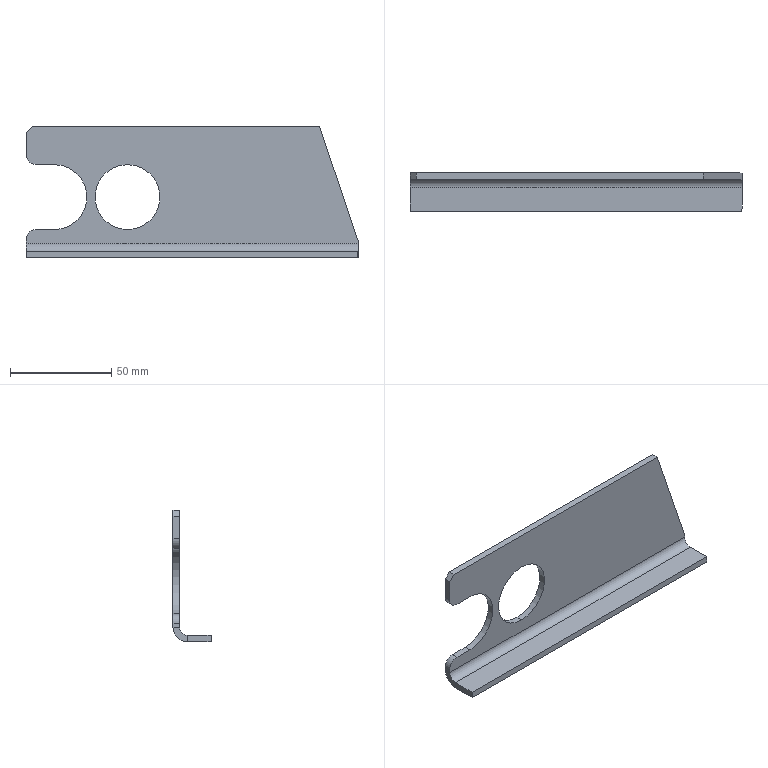Part | SolidWorks | features ICE 3, Fillet 2, BreakCorner 1, EdgeFlange 1, FlatPattern 1, SMBaseFlange 1, SheetMetal 1 | 1 solid | 25 faces | box 163.6 x 18.8 x 65 mm | volume 33886 mm3 | plane 17 | cylinder 8 | commonest cylinder face diameters 32 x3 10 x2 8 x1 14.4 x1 24 x1
STEP:
#1=CARTESIAN_POINT('',(-31.8,-3.2,-18.5));
#2=VERTEX_POINT('',#1);
#3=CARTESIAN_POINT('',(-31.8,-3.2,13.5));
#4=VERTEX_POINT('',#3);
#5=CARTESIAN_POINT('',(-31.8,-3.2,-2.5));
#6=DIRECTION('',(0.,1.,0.));
#7=DIRECTION('',(0.,0.,1.));
#8=AXIS2_PLACEMENT_3D('',#5,#6,#7);
#9=CIRCLE('',#8,16.);
#10=EDGE_CURVE('',#2,#4,#9,.T.);
#11=ORIENTED_EDGE('',*,*,#10,.F.);
#12=CARTESIAN_POINT('',(-31.8,0.,-18.5));
#13=VERTEX_POINT('',#12);
#14=CARTESIAN_POINT('',(-31.8,-10.,-18.5));
#15=DIRECTION('',(0.,1.,0.));
#16=VECTOR('',#15,1000.);
#17=LINE('',#14,#16);
#18=EDGE_CURVE('',#2,#13,#17,.T.);
#19=ORIENTED_EDGE('',*,*,#18,.T.);
#20=CARTESIAN_POINT('',(-31.8,0.,13.5));
#21=VERTEX_POINT('',#20);
#22=CARTESIAN_POINT('',(-31.8,0.,-2.5));
#23=DIRECTION('',(0.,1.,0.));
#24=DIRECTION('',(0.,0.,1.));
#25=AXIS2_PLACEMENT_3D('',#22,#23,#24);
#26=CIRCLE('',#25,16.);
#27=EDGE_CURVE('',#13,#21,#26,.T.);
#28=ORIENTED_EDGE('',*,*,#27,.T.);
#29=CARTESIAN_POINT('',(-31.8,-10.,13.5));
#30=DIRECTION('',(0.,1.,0.));
#31=VECTOR('',#30,1000.);
#32=LINE('',#29,#31);
#33=EDGE_CURVE('',#4,#21,#32,.T.);
#34=ORIENTED_EDGE('',*,*,#33,.F.);
#35=EDGE_LOOP('',(#11,#19,#28,#34));
#36=FACE_OUTER_BOUND('',#35,.T.);
#37=CARTESIAN_POINT('',(-31.8,-10.,-2.5));
#38=DIRECTION('',(0.,1.,0.));
#39=DIRECTION('',(0.,0.,1.));
#40=AXIS2_PLACEMENT_3D('',#37,#38,#39);
#41=CYLINDRICAL_SURFACE('',#40,16.);
#42=ADVANCED_FACE('',(#36),#41,.F.);
#43=CARTESIAN_POINT('',(81.8,0.,-23.7));
#44=VERTEX_POINT('',#43);
#45=CARTESIAN_POINT('',(81.8,0.,-25.3));
#46=VERTEX_POINT('',#45);
#47=CARTESIAN_POINT('',(81.8,0.,-32.5));
#48=DIRECTION('',(0.,0.,-1.));
#49=VECTOR('',#48,1000.);
#50=LINE('',#47,#49);
#51=EDGE_CURVE('',#44,#46,#50,.T.);
#52=ORIENTED_EDGE('',*,*,#51,.F.);
#53=CARTESIAN_POINT('',(81.8,-3.2,-23.7));
#54=VERTEX_POINT('',#53);
#55=CARTESIAN_POINT('',(81.8,0.,-23.7));
#56=DIRECTION('',(0.,-1.,0.));
#57=VECTOR('',#56,1000.);
#58=LINE('',#55,#57);
#59=EDGE_CURVE('',#44,#54,#58,.T.);
#60=ORIENTED_EDGE('',*,*,#59,.T.);
#61=CARTESIAN_POINT('',(81.8,-3.2,-25.3));
#62=VERTEX_POINT('',#61);
#63=CARTESIAN_POINT('',(81.8,-3.2,-32.5));
#64=DIRECTION('',(0.,0.,-1.));
#65=VECTOR('',#64,1000.);
#66=LINE('',#63,#65);
#67=EDGE_CURVE('',#54,#62,#66,.T.);
#68=ORIENTED_EDGE('',*,*,#67,.T.);
#69=CARTESIAN_POINT('',(81.8,-3.2,-25.3));
#70=DIRECTION('',(0.,1.,0.));
#71=VECTOR('',#70,1000.);
#72=LINE('',#69,#71);
#73=EDGE_CURVE('',#62,#46,#72,.T.);
#74=ORIENTED_EDGE('',*,*,#73,.T.);
#75=EDGE_LOOP('',(#52,#60,#68,#74));
#76=FACE_OUTER_BOUND('',#75,.T.);
#77=CARTESIAN_POINT('',(81.8,-3.2,-32.5));
#78=DIRECTION('',(1.,0.,0.));
#79=DIRECTION('',(0.,0.,-1.));
#80=AXIS2_PLACEMENT_3D('',#77,#78,#79);
#81=PLANE('',#80);
#82=ADVANCED_FACE('',(#76),#81,.T.);
#83=CARTESIAN_POINT('',(-31.8,-3.2,-2.5));
#84=DIRECTION('',(0.,1.,0.));
#85=DIRECTION('',(0.,0.,1.));
#86=AXIS2_PLACEMENT_3D('',#83,#84,#85);
#87=CIRCLE('',#86,16.);
#88=EDGE_CURVE('',#4,#2,#87,.T.);
#89=ORIENTED_EDGE('',*,*,#88,.T.);
#90=ORIENTED_EDGE('',*,*,#10,.T.);
#91=EDGE_LOOP('',(#89,#90));
#92=FACE_BOUND('',#91,.T.);
#93=CARTESIAN_POINT('',(-78.8,-3.2,32.5));
#94=VERTEX_POINT('',#93);
#95=CARTESIAN_POINT('',(62.8,-3.2,32.5));
#96=VERTEX_POINT('',#95);
#97=CARTESIAN_POINT('',(-81.8,-3.2,32.5));
#98=DIRECTION('',(1.,0.,0.));
#99=VECTOR('',#98,1000.);
#100=LINE('',#97,#99);
#101=EDGE_CURVE('',#94,#96,#100,.T.);
#102=ORIENTED_EDGE('',*,*,#101,.F.);
#103=CARTESIAN_POINT('',(-81.8,-3.2,29.5));
#104=VERTEX_POINT('',#103);
#105=CARTESIAN_POINT('',(-81.8,-3.2,29.5));
#106=DIRECTION('',(-0.7071,0.,-0.7071));
#107=VECTOR('',#106,1000.);
#108=LINE('',#105,#107);
#109=EDGE_CURVE('',#94,#104,#108,.T.);
#110=ORIENTED_EDGE('',*,*,#109,.T.);
#111=CARTESIAN_POINT('',(-81.8,-3.2,18.5));
#112=VERTEX_POINT('',#111);
#113=CARTESIAN_POINT('',(-81.8,-3.2,-32.5));
#114=DIRECTION('',(0.,0.,1.));
#115=VECTOR('',#114,1000.);
#116=LINE('',#113,#115);
#117=EDGE_CURVE('',#112,#104,#116,.T.);
#118=ORIENTED_EDGE('',*,*,#117,.F.);
#119=CARTESIAN_POINT('',(-76.8,-3.2,13.5));
#120=VERTEX_POINT('',#119);
#121=CARTESIAN_POINT('',(-76.8,-3.2,18.5));
#122=DIRECTION('',(0.,-1.,0.));
#123=DIRECTION('',(0.,0.,1.));
#124=AXIS2_PLACEMENT_3D('',#121,#122,#123);
#125=CIRCLE('',#124,5.);
#126=EDGE_CURVE('',#112,#120,#125,.T.);
#127=ORIENTED_EDGE('',*,*,#126,.T.);
#128=CARTESIAN_POINT('',(-67.8,-3.2,13.5));
#129=VERTEX_POINT('',#128);
#130=CARTESIAN_POINT('',(0.,-3.2,13.5));
#131=DIRECTION('',(1.,0.,0.));
#132=VECTOR('',#131,1000.);
#133=LINE('',#130,#132);
#134=EDGE_CURVE('',#120,#129,#133,.T.);
#135=ORIENTED_EDGE('',*,*,#134,.T.);
#136=CARTESIAN_POINT('',(-67.8,-3.2,-18.5));
#137=VERTEX_POINT('',#136);
#138=CARTESIAN_POINT('',(-67.8,-3.2,-2.5));
#139=DIRECTION('',(0.,1.,0.));
#140=DIRECTION('',(0.,0.,1.));
#141=AXIS2_PLACEMENT_3D('',#138,#139,#140);
#142=CIRCLE('',#141,16.);
#143=EDGE_CURVE('',#129,#137,#142,.T.);
#144=ORIENTED_EDGE('',*,*,#143,.T.);
#145=CARTESIAN_POINT('',(-76.8,-3.2,-18.5));
#146=VERTEX_POINT('',#145);
#147=CARTESIAN_POINT('',(0.,-3.2,-18.5));
#148=DIRECTION('',(-1.,0.,0.));
#149=VECTOR('',#148,1000.);
#150=LINE('',#147,#149);
#151=EDGE_CURVE('',#137,#146,#150,.T.);
#152=ORIENTED_EDGE('',*,*,#151,.T.);
#153=CARTESIAN_POINT('',(-81.8,-3.2,-23.5));
#154=VERTEX_POINT('',#153);
#155=CARTESIAN_POINT('',(-76.8,-3.2,-23.5));
#156=DIRECTION('',(0.,-1.,0.));
#157=DIRECTION('',(0.,0.,1.));
#158=AXIS2_PLACEMENT_3D('',#155,#156,#157);
#159=CIRCLE('',#158,5.);
#160=EDGE_CURVE('',#146,#154,#159,.T.);
#161=ORIENTED_EDGE('',*,*,#160,.T.);
#162=CARTESIAN_POINT('',(-81.8,-3.2,-25.3));
#163=VERTEX_POINT('',#162);
#164=CARTESIAN_POINT('',(-81.8,-3.2,-32.5));
#165=DIRECTION('',(0.,0.,1.));
#166=VECTOR('',#165,1000.);
#167=LINE('',#164,#166);
#168=EDGE_CURVE('',#163,#154,#167,.T.);
#169=ORIENTED_EDGE('',*,*,#168,.F.);
#170=CARTESIAN_POINT('',(81.8,-3.2,-25.3));
#171=DIRECTION('',(-1.,0.,0.));
#172=VECTOR('',#171,1000.);
#173=LINE('',#170,#172);
#174=EDGE_CURVE('',#62,#163,#173,.T.);
#175=ORIENTED_EDGE('',*,*,#174,.F.);
#176=ORIENTED_EDGE('',*,*,#67,.F.);
#177=CARTESIAN_POINT('',(66.219,-3.2,22.387));
#178=DIRECTION('',(0.3203,0.,-0.9473));
#179=VECTOR('',#178,1000.);
#180=LINE('',#177,#179);
#181=EDGE_CURVE('',#96,#54,#180,.T.);
#182=ORIENTED_EDGE('',*,*,#181,.F.);
#183=EDGE_LOOP('',(#102,#110,#118,#127,#135,#144,#152,#161,#169,#175,#176,#182));
#184=FACE_OUTER_BOUND('',#183,.T.);
#185=CARTESIAN_POINT('',(0.,-3.2,0.));
#186=DIRECTION('',(0.,1.,0.));
#187=DIRECTION('',(0.,0.,1.));
#188=AXIS2_PLACEMENT_3D('',#185,#186,#187);
#189=PLANE('',#188);
#190=ADVANCED_FACE('',(#92,#184),#189,.F.);
#191=CARTESIAN_POINT('',(-31.8,0.,-2.5));
#192=DIRECTION('',(0.,1.,0.));
#193=DIRECTION('',(0.,0.,1.));
#194=AXIS2_PLACEMENT_3D('',#191,#192,#193);
#195=CIRCLE('',#194,16.);
#196=EDGE_CURVE('',#21,#13,#195,.T.);
#197=ORIENTED_EDGE('',*,*,#196,.F.);
#198=ORIENTED_EDGE('',*,*,#27,.F.);
#199=EDGE_LOOP('',(#197,#198));
#200=FACE_BOUND('',#199,.T.);
#201=CARTESIAN_POINT('',(-81.8,0.,18.5));
#202=VERTEX_POINT('',#201);
#203=CARTESIAN_POINT('',(-81.8,0.,29.5));
#204=VERTEX_POINT('',#203);
#205=CARTESIAN_POINT('',(-81.8,0.,-32.5));
#206=DIRECTION('',(0.,0.,1.));
#207=VECTOR('',#206,1000.);
#208=LINE('',#205,#207);
#209=EDGE_CURVE('',#202,#204,#208,.T.);
#210=ORIENTED_EDGE('',*,*,#209,.T.);
#211=CARTESIAN_POINT('',(-78.8,0.,32.5));
#212=VERTEX_POINT('',#211);
#213=CARTESIAN_POINT('',(-55.65,0.,55.65));
#214=DIRECTION('',(0.7071,0.,0.7071));
#215=VECTOR('',#214,1000.);
#216=LINE('',#213,#215);
#217=EDGE_CURVE('',#204,#212,#216,.T.);
#218=ORIENTED_EDGE('',*,*,#217,.T.);
#219=CARTESIAN_POINT('',(62.8,0.,32.5));
#220=VERTEX_POINT('',#219);
#221=CARTESIAN_POINT('',(-81.8,0.,32.5));
#222=DIRECTION('',(1.,0.,0.));
#223=VECTOR('',#222,1000.);
#224=LINE('',#221,#223);
#225=EDGE_CURVE('',#212,#220,#224,.T.);
#226=ORIENTED_EDGE('',*,*,#225,.T.);
#227=CARTESIAN_POINT('',(66.219,0.,22.387));
#228=DIRECTION('',(0.3203,0.,-0.9473));
#229=VECTOR('',#228,1000.);
#230=LINE('',#227,#229);
#231=EDGE_CURVE('',#220,#44,#230,.T.);
#232=ORIENTED_EDGE('',*,*,#231,.T.);
#233=ORIENTED_EDGE('',*,*,#51,.T.);
#234=CARTESIAN_POINT('',(-81.8,0.,-25.3));
#235=VERTEX_POINT('',#234);
#236=CARTESIAN_POINT('',(81.8,0.,-25.3));
#237=DIRECTION('',(-1.,0.,0.));
#238=VECTOR('',#237,1000.);
#239=LINE('',#236,#238);
#240=EDGE_CURVE('',#46,#235,#239,.T.);
#241=ORIENTED_EDGE('',*,*,#240,.T.);
#242=CARTESIAN_POINT('',(-81.8,0.,-23.5));
#243=VERTEX_POINT('',#242);
#244=CARTESIAN_POINT('',(-81.8,0.,-32.5));
#245=DIRECTION('',(0.,0.,1.));
#246=VECTOR('',#245,1000.);
#247=LINE('',#244,#246);
#248=EDGE_CURVE('',#235,#243,#247,.T.);
#249=ORIENTED_EDGE('',*,*,#248,.T.);
#250=CARTESIAN_POINT('',(-76.8,0.,-18.5));
#251=VERTEX_POINT('',#250);
#252=CARTESIAN_POINT('',(-76.8,0.,-23.5));
#253=DIRECTION('',(0.,1.,0.));
#254=DIRECTION('',(0.,0.,1.));
#255=AXIS2_PLACEMENT_3D('',#252,#253,#254);
#256=CIRCLE('',#255,5.);
#257=EDGE_CURVE('',#243,#251,#256,.T.);
#258=ORIENTED_EDGE('',*,*,#257,.T.);
#259=CARTESIAN_POINT('',(-67.8,0.,-18.5));
#260=VERTEX_POINT('',#259);
#261=CARTESIAN_POINT('',(-67.8,0.,-18.5));
#262=DIRECTION('',(-1.,0.,0.));
#263=VECTOR('',#262,1000.);
#264=LINE('',#261,#263);
#265=EDGE_CURVE('',#260,#251,#264,.T.);
#266=ORIENTED_EDGE('',*,*,#265,.F.);
#267=CARTESIAN_POINT('',(-67.8,0.,13.5));
#268=VERTEX_POINT('',#267);
#269=CARTESIAN_POINT('',(-67.8,0.,-2.5));
#270=DIRECTION('',(0.,1.,0.));
#271=DIRECTION('',(0.,0.,1.));
#272=AXIS2_PLACEMENT_3D('',#269,#270,#271);
#273=CIRCLE('',#272,16.);
#274=EDGE_CURVE('',#268,#260,#273,.T.);
#275=ORIENTED_EDGE('',*,*,#274,.F.);
#276=CARTESIAN_POINT('',(-76.8,0.,13.5));
#277=VERTEX_POINT('',#276);
#278=CARTESIAN_POINT('',(-67.8,0.,13.5));
#279=DIRECTION('',(1.,0.,0.));
#280=VECTOR('',#279,1000.);
#281=LINE('',#278,#280);
#282=EDGE_CURVE('',#277,#268,#281,.T.);
#283=ORIENTED_EDGE('',*,*,#282,.F.);
#284=CARTESIAN_POINT('',(-76.8,0.,18.5));
#285=DIRECTION('',(0.,1.,0.));
#286=DIRECTION('',(0.,0.,1.));
#287=AXIS2_PLACEMENT_3D('',#284,#285,#286);
#288=CIRCLE('',#287,5.);
#289=EDGE_CURVE('',#277,#202,#288,.T.);
#290=ORIENTED_EDGE('',*,*,#289,.T.);
#291=EDGE_LOOP('',(#210,#218,#226,#232,#233,#241,#249,#258,#266,#275,#283,#290));
#292=FACE_OUTER_BOUND('',#291,.T.);
#293=CARTESIAN_POINT('',(0.,0.,0.));
#294=DIRECTION('',(0.,1.,0.));
#295=DIRECTION('',(0.,0.,1.));
#296=AXIS2_PLACEMENT_3D('',#293,#294,#295);
#297=PLANE('',#296);
#298=ADVANCED_FACE('',(#200,#292),#297,.T.);
#299=ORIENTED_EDGE('',*,*,#225,.F.);
#300=CARTESIAN_POINT('',(-78.8,-3.2,32.5));
#301=DIRECTION('',(0.,-1.,0.));
#302=VECTOR('',#301,1000.);
#303=LINE('',#300,#302);
#304=EDGE_CURVE('',#212,#94,#303,.T.);
#305=ORIENTED_EDGE('',*,*,#304,.T.);
#306=ORIENTED_EDGE('',*,*,#101,.T.);
#307=CARTESIAN_POINT('',(62.8,0.,32.5));
#308=DIRECTION('',(0.,-1.,0.));
#309=VECTOR('',#308,1000.);
#310=LINE('',#307,#309);
#311=EDGE_CURVE('',#220,#96,#310,.T.);
#312=ORIENTED_EDGE('',*,*,#311,.F.);
#313=EDGE_LOOP('',(#299,#305,#306,#312));
#314=FACE_OUTER_BOUND('',#313,.T.);
#315=CARTESIAN_POINT('',(-81.8,-3.2,32.5));
#316=DIRECTION('',(0.,0.,1.));
#317=DIRECTION('',(1.,0.,0.));
#318=AXIS2_PLACEMENT_3D('',#315,#316,#317);
#319=PLANE('',#318);
#320=ADVANCED_FACE('',(#314),#319,.T.);
#321=ORIENTED_EDGE('',*,*,#117,.T.);
#322=CARTESIAN_POINT('',(-81.8,-3.2,29.5));
#323=DIRECTION('',(0.,1.,0.));
#324=VECTOR('',#323,1000.);
#325=LINE('',#322,#324);
#326=EDGE_CURVE('',#104,#204,#325,.T.);
#327=ORIENTED_EDGE('',*,*,#326,.T.);
#328=ORIENTED_EDGE('',*,*,#209,.F.);
#329=CARTESIAN_POINT('',(-81.8,-3.2,18.5));
#330=DIRECTION('',(0.,-1.,0.));
#331=VECTOR('',#330,1000.);
#332=LINE('',#329,#331);
#333=EDGE_CURVE('',#202,#112,#332,.T.);
#334=ORIENTED_EDGE('',*,*,#333,.T.);
#335=EDGE_LOOP('',(#321,#327,#328,#334));
#336=FACE_OUTER_BOUND('',#335,.T.);
#337=CARTESIAN_POINT('',(-81.8,-3.2,-32.5));
#338=DIRECTION('',(-1.,0.,0.));
#339=DIRECTION('',(0.,0.,1.));
#340=AXIS2_PLACEMENT_3D('',#337,#338,#339);
#341=PLANE('',#340);
#342=ADVANCED_FACE('',(#336),#341,.T.);
#343=CARTESIAN_POINT('',(81.8,-17.254,-29.3));
#344=VERTEX_POINT('',#343);
#345=CARTESIAN_POINT('',(81.8,-7.2,-29.3));
#346=VERTEX_POINT('',#345);
#347=CARTESIAN_POINT('',(81.8,0.,-29.3));
#348=DIRECTION('',(0.,1.,0.));
#349=VECTOR('',#348,1000.);
#350=LINE('',#347,#349);
#351=EDGE_CURVE('',#344,#346,#350,.T.);
#352=ORIENTED_EDGE('',*,*,#351,.F.);
#353=CARTESIAN_POINT('',(81.8,-17.254,-32.5));
#354=VERTEX_POINT('',#353);
#355=CARTESIAN_POINT('',(81.8,-17.254,-32.5));
#356=DIRECTION('',(0.,0.,-1.));
#357=VECTOR('',#356,1000.);
#358=LINE('',#355,#357);
#359=EDGE_CURVE('',#344,#354,#358,.T.);
#360=ORIENTED_EDGE('',*,*,#359,.T.);
#361=CARTESIAN_POINT('',(81.8,-7.2,-32.5));
#362=VERTEX_POINT('',#361);
#363=CARTESIAN_POINT('',(81.8,-18.8,-32.5));
#364=DIRECTION('',(0.,1.,0.));
#365=VECTOR('',#364,1000.);
#366=LINE('',#363,#365);
#367=EDGE_CURVE('',#354,#362,#366,.T.);
#368=ORIENTED_EDGE('',*,*,#367,.T.);
#369=CARTESIAN_POINT('',(81.8,-7.2,-29.3));
#370=DIRECTION('',(0.,0.,-1.));
#371=VECTOR('',#370,1000.);
#372=LINE('',#369,#371);
#373=EDGE_CURVE('',#346,#362,#372,.T.);
#374=ORIENTED_EDGE('',*,*,#373,.F.);
#375=EDGE_LOOP('',(#352,#360,#368,#374));
#376=FACE_OUTER_BOUND('',#375,.T.);
#377=CARTESIAN_POINT('',(81.8,-18.8,-32.5));
#378=DIRECTION('',(1.,0.,0.));
#379=DIRECTION('',(0.,0.,-1.));
#380=AXIS2_PLACEMENT_3D('',#377,#378,#379);
#381=PLANE('',#380);
#382=ADVANCED_FACE('',(#376),#381,.T.);
#383=ORIENTED_EDGE('',*,*,#367,.F.);
#384=CARTESIAN_POINT('',(81.7,-18.8,-32.5));
#385=VERTEX_POINT('',#384);
#386=CARTESIAN_POINT('',(69.8,-17.254,-32.5));
#387=DIRECTION('',(0.,0.,-1.));
#388=DIRECTION('',(0.,-1.,0.));
#389=AXIS2_PLACEMENT_3D('',#386,#387,#388);
#390=CIRCLE('',#389,12.);
#391=EDGE_CURVE('',#354,#385,#390,.T.);
#392=ORIENTED_EDGE('',*,*,#391,.T.);
#393=CARTESIAN_POINT('',(-81.8,-18.8,-32.5));
#394=VERTEX_POINT('',#393);
#395=CARTESIAN_POINT('',(-81.8,-18.8,-32.5));
#396=DIRECTION('',(1.,0.,0.));
#397=VECTOR('',#396,1000.);
#398=LINE('',#395,#397);
#399=EDGE_CURVE('',#394,#385,#398,.T.);
#400=ORIENTED_EDGE('',*,*,#399,.F.);
#401=CARTESIAN_POINT('',(-81.8,-7.2,-32.5));
#402=VERTEX_POINT('',#401);
#403=CARTESIAN_POINT('',(-81.8,-3.2,-32.5));
#404=DIRECTION('',(0.,-1.,0.));
#405=VECTOR('',#404,1000.);
#406=LINE('',#403,#405);
#407=EDGE_CURVE('',#402,#394,#406,.T.);
#408=ORIENTED_EDGE('',*,*,#407,.F.);
#409=CARTESIAN_POINT('',(-81.8,-7.2,-32.5));
#410=DIRECTION('',(-1.,0.,0.));
#411=VECTOR('',#410,1000.);
#412=LINE('',#409,#411);
#413=EDGE_CURVE('',#362,#402,#412,.T.);
#414=ORIENTED_EDGE('',*,*,#413,.F.);
#415=EDGE_LOOP('',(#383,#392,#400,#408,#414));
#416=FACE_OUTER_BOUND('',#415,.T.);
#417=CARTESIAN_POINT('',(0.,0.,-32.5));
#418=DIRECTION('',(0.,0.,1.));
#419=DIRECTION('',(0.,-1.,0.));
#420=AXIS2_PLACEMENT_3D('',#417,#418,#419);
#421=PLANE('',#420);
#422=ADVANCED_FACE('',(#416),#421,.F.);
#423=CARTESIAN_POINT('',(-81.8,-18.8,-29.3));
#424=VERTEX_POINT('',#423);
#425=CARTESIAN_POINT('',(81.7,-18.8,-29.3));
#426=VERTEX_POINT('',#425);
#427=CARTESIAN_POINT('',(0.,-18.8,-29.3));
#428=DIRECTION('',(1.,0.,0.));
#429=VECTOR('',#428,1000.);
#430=LINE('',#427,#429);
#431=EDGE_CURVE('',#424,#426,#430,.T.);
#432=ORIENTED_EDGE('',*,*,#431,.T.);
#433=CARTESIAN_POINT('',(69.8,-17.254,-29.3));
#434=DIRECTION('',(0.,0.,1.));
#435=DIRECTION('',(0.,-1.,0.));
#436=AXIS2_PLACEMENT_3D('',#433,#434,#435);
#437=CIRCLE('',#436,12.);
#438=EDGE_CURVE('',#426,#344,#437,.T.);
#439=ORIENTED_EDGE('',*,*,#438,.T.);
#440=ORIENTED_EDGE('',*,*,#351,.T.);
#441=CARTESIAN_POINT('',(-81.8,-7.2,-29.3));
#442=VERTEX_POINT('',#441);
#443=CARTESIAN_POINT('',(-81.8,-7.2,-29.3));
#444=DIRECTION('',(1.,0.,0.));
#445=VECTOR('',#444,1000.);
#446=LINE('',#443,#445);
#447=EDGE_CURVE('',#442,#346,#446,.T.);
#448=ORIENTED_EDGE('',*,*,#447,.F.);
#449=CARTESIAN_POINT('',(-81.8,0.,-29.3));
#450=DIRECTION('',(0.,-1.,0.));
#451=VECTOR('',#450,1000.);
#452=LINE('',#449,#451);
#453=EDGE_CURVE('',#442,#424,#452,.T.);
#454=ORIENTED_EDGE('',*,*,#453,.T.);
#455=EDGE_LOOP('',(#432,#439,#440,#448,#454));
#456=FACE_OUTER_BOUND('',#455,.T.);
#457=CARTESIAN_POINT('',(0.,0.,-29.3));
#458=DIRECTION('',(0.,0.,1.));
#459=DIRECTION('',(0.,-1.,0.));
#460=AXIS2_PLACEMENT_3D('',#457,#458,#459);
#461=PLANE('',#460);
#462=ADVANCED_FACE('',(#456),#461,.T.);
#463=ORIENTED_EDGE('',*,*,#399,.T.);
#464=CARTESIAN_POINT('',(81.7,-18.8,-32.5));
#465=DIRECTION('',(0.,0.,1.));
#466=VECTOR('',#465,1000.);
#467=LINE('',#464,#466);
#468=EDGE_CURVE('',#385,#426,#467,.T.);
#469=ORIENTED_EDGE('',*,*,#468,.T.);
#470=ORIENTED_EDGE('',*,*,#431,.F.);
#471=CARTESIAN_POINT('',(-81.8,-18.8,-32.5));
#472=DIRECTION('',(0.,0.,1.));
#473=VECTOR('',#472,1000.);
#474=LINE('',#471,#473);
#475=EDGE_CURVE('',#394,#424,#474,.T.);
#476=ORIENTED_EDGE('',*,*,#475,.F.);
#477=EDGE_LOOP('',(#463,#469,#470,#476));
#478=FACE_OUTER_BOUND('',#477,.T.);
#479=CARTESIAN_POINT('',(-81.8,-18.8,-32.5));
#480=DIRECTION('',(0.,-1.,0.));
#481=DIRECTION('',(0.,0.,-1.));
#482=AXIS2_PLACEMENT_3D('',#479,#480,#481);
#483=PLANE('',#482);
#484=ADVANCED_FACE('',(#478),#483,.T.);
#485=ORIENTED_EDGE('',*,*,#168,.T.);
#486=CARTESIAN_POINT('',(-81.8,0.,-23.5));
#487=DIRECTION('',(0.,1.,0.));
#488=VECTOR('',#487,1000.);
#489=LINE('',#486,#488);
#490=EDGE_CURVE('',#154,#243,#489,.T.);
#491=ORIENTED_EDGE('',*,*,#490,.T.);
#492=ORIENTED_EDGE('',*,*,#248,.F.);
#493=CARTESIAN_POINT('',(-81.8,-3.2,-25.3));
#494=DIRECTION('',(0.,1.,0.));
#495=VECTOR('',#494,1000.);
#496=LINE('',#493,#495);
#497=EDGE_CURVE('',#163,#235,#496,.T.);
#498=ORIENTED_EDGE('',*,*,#497,.F.);
#499=EDGE_LOOP('',(#485,#491,#492,#498));
#500=FACE_OUTER_BOUND('',#499,.T.);
#501=CARTESIAN_POINT('',(-81.8,-3.2,-32.5));
#502=DIRECTION('',(-1.,0.,0.));
#503=DIRECTION('',(0.,0.,1.));
#504=AXIS2_PLACEMENT_3D('',#501,#502,#503);
#505=PLANE('',#504);
#506=ADVANCED_FACE('',(#500),#505,.T.);
#507=CARTESIAN_POINT('',(-81.8,-7.2,-32.5));
#508=DIRECTION('',(0.,0.,-1.));
#509=VECTOR('',#508,1000.);
#510=LINE('',#507,#509);
#511=EDGE_CURVE('',#442,#402,#510,.T.);
#512=ORIENTED_EDGE('',*,*,#511,.F.);
#513=CARTESIAN_POINT('',(-81.8,-7.2,-25.3));
#514=DIRECTION('',(-1.,0.,0.));
#515=DIRECTION('',(0.,0.,-1.));
#516=AXIS2_PLACEMENT_3D('',#513,#514,#515);
#517=CIRCLE('',#516,4.);
#518=EDGE_CURVE('',#163,#442,#517,.T.);
#519=ORIENTED_EDGE('',*,*,#518,.F.);
#520=ORIENTED_EDGE('',*,*,#497,.T.);
#521=CARTESIAN_POINT('',(-81.8,-7.2,-25.3));
#522=DIRECTION('',(-1.,0.,0.));
#523=DIRECTION('',(0.,0.,-1.));
#524=AXIS2_PLACEMENT_3D('',#521,#522,#523);
#525=CIRCLE('',#524,7.2);
#526=EDGE_CURVE('',#235,#402,#525,.T.);
#527=ORIENTED_EDGE('',*,*,#526,.T.);
#528=EDGE_LOOP('',(#512,#519,#520,#527));
#529=FACE_OUTER_BOUND('',#528,.T.);
#530=CARTESIAN_POINT('',(-81.8,-7.2,-25.3));
#531=DIRECTION('',(-1.,0.,0.));
#532=DIRECTION('',(0.,0.,1.));
#533=AXIS2_PLACEMENT_3D('',#530,#531,#532);
#534=PLANE('',#533);
#535=ADVANCED_FACE('',(#529),#534,.T.);
#536=CARTESIAN_POINT('',(81.8,-7.2,-25.3));
#537=DIRECTION('',(1.,0.,0.));
#538=DIRECTION('',(0.,0.,-1.));
#539=AXIS2_PLACEMENT_3D('',#536,#537,#538);
#540=CIRCLE('',#539,4.);
#541=EDGE_CURVE('',#346,#62,#540,.T.);
#542=ORIENTED_EDGE('',*,*,#541,.F.);
#543=ORIENTED_EDGE('',*,*,#373,.T.);
#544=CARTESIAN_POINT('',(81.8,-7.2,-25.3));
#545=DIRECTION('',(1.,0.,0.));
#546=DIRECTION('',(0.,0.,-1.));
#547=AXIS2_PLACEMENT_3D('',#544,#545,#546);
#548=CIRCLE('',#547,7.2);
#549=EDGE_CURVE('',#362,#46,#548,.T.);
#550=ORIENTED_EDGE('',*,*,#549,.T.);
#551=ORIENTED_EDGE('',*,*,#73,.F.);
#552=EDGE_LOOP('',(#542,#543,#550,#551));
#553=FACE_OUTER_BOUND('',#552,.T.);
#554=CARTESIAN_POINT('',(81.8,-7.2,-25.3));
#555=DIRECTION('',(-1.,0.,0.));
#556=DIRECTION('',(0.,0.,1.));
#557=AXIS2_PLACEMENT_3D('',#554,#555,#556);
#558=PLANE('',#557);
#559=ADVANCED_FACE('',(#553),#558,.F.);
#560=ORIENTED_EDGE('',*,*,#240,.F.);
#561=ORIENTED_EDGE('',*,*,#549,.F.);
#562=ORIENTED_EDGE('',*,*,#413,.T.);
#563=ORIENTED_EDGE('',*,*,#526,.F.);
#564=EDGE_LOOP('',(#560,#561,#562,#563));
#565=FACE_OUTER_BOUND('',#564,.T.);
#566=CARTESIAN_POINT('',(81.8,-7.2,-25.3));
#567=DIRECTION('',(1.,0.,0.));
#568=DIRECTION('',(0.,0.,-1.));
#569=AXIS2_PLACEMENT_3D('',#566,#567,#568);
#570=CYLINDRICAL_SURFACE('',#569,7.2);
#571=ADVANCED_FACE('',(#565),#570,.T.);
#572=ORIENTED_EDGE('',*,*,#174,.T.);
#573=ORIENTED_EDGE('',*,*,#518,.T.);
#574=ORIENTED_EDGE('',*,*,#447,.T.);
#575=ORIENTED_EDGE('',*,*,#541,.T.);
#576=EDGE_LOOP('',(#572,#573,#574,#575));
#577=FACE_OUTER_BOUND('',#576,.T.);
#578=CARTESIAN_POINT('',(81.8,-7.2,-25.3));
#579=DIRECTION('',(1.,0.,0.));
#580=DIRECTION('',(0.,0.,-1.));
#581=AXIS2_PLACEMENT_3D('',#578,#579,#580);
#582=CYLINDRICAL_SURFACE('',#581,4.);
#583=ADVANCED_FACE('',(#577),#582,.F.);
#584=ORIENTED_EDGE('',*,*,#453,.F.);
#585=ORIENTED_EDGE('',*,*,#511,.T.);
#586=ORIENTED_EDGE('',*,*,#407,.T.);
#587=ORIENTED_EDGE('',*,*,#475,.T.);
#588=EDGE_LOOP('',(#584,#585,#586,#587));
#589=FACE_OUTER_BOUND('',#588,.T.);
#590=CARTESIAN_POINT('',(-81.8,-3.2,-32.5));
#591=DIRECTION('',(-1.,0.,0.));
#592=DIRECTION('',(0.,0.,1.));
#593=AXIS2_PLACEMENT_3D('',#590,#591,#592);
#594=PLANE('',#593);
#595=ADVANCED_FACE('',(#589),#594,.T.);
#596=CARTESIAN_POINT('',(-67.8,-10.,13.5));
#597=DIRECTION('',(0.,1.,0.));
#598=VECTOR('',#597,1000.);
#599=LINE('',#596,#598);
#600=EDGE_CURVE('',#129,#268,#599,.T.);
#601=ORIENTED_EDGE('',*,*,#600,.T.);
#602=ORIENTED_EDGE('',*,*,#274,.T.);
#603=CARTESIAN_POINT('',(-67.8,-10.,-18.5));
#604=DIRECTION('',(0.,1.,0.));
#605=VECTOR('',#604,1000.);
#606=LINE('',#603,#605);
#607=EDGE_CURVE('',#137,#260,#606,.T.);
#608=ORIENTED_EDGE('',*,*,#607,.F.);
#609=ORIENTED_EDGE('',*,*,#143,.F.);
#610=EDGE_LOOP('',(#601,#602,#608,#609));
#611=FACE_OUTER_BOUND('',#610,.T.);
#612=CARTESIAN_POINT('',(-67.8,-10.,-2.5));
#613=DIRECTION('',(0.,1.,0.));
#614=DIRECTION('',(0.,0.,1.));
#615=AXIS2_PLACEMENT_3D('',#612,#613,#614);
#616=CYLINDRICAL_SURFACE('',#615,16.);
#617=ADVANCED_FACE('',(#611),#616,.F.);
#618=ORIENTED_EDGE('',*,*,#134,.F.);
#619=CARTESIAN_POINT('',(-76.8,0.,13.5));
#620=DIRECTION('',(0.,1.,0.));
#621=VECTOR('',#620,1000.);
#622=LINE('',#619,#621);
#623=EDGE_CURVE('',#120,#277,#622,.T.);
#624=ORIENTED_EDGE('',*,*,#623,.T.);
#625=ORIENTED_EDGE('',*,*,#282,.T.);
#626=ORIENTED_EDGE('',*,*,#600,.F.);
#627=EDGE_LOOP('',(#618,#624,#625,#626));
#628=FACE_OUTER_BOUND('',#627,.T.);
#629=CARTESIAN_POINT('',(-67.8,-10.,13.5));
#630=DIRECTION('',(0.,0.,1.));
#631=DIRECTION('',(1.,0.,0.));
#632=AXIS2_PLACEMENT_3D('',#629,#630,#631);
#633=PLANE('',#632);
#634=ADVANCED_FACE('',(#628),#633,.F.);
#635=ORIENTED_EDGE('',*,*,#265,.T.);
#636=CARTESIAN_POINT('',(-76.8,-3.2,-18.5));
#637=DIRECTION('',(0.,-1.,0.));
#638=VECTOR('',#637,1000.);
#639=LINE('',#636,#638);
#640=EDGE_CURVE('',#251,#146,#639,.T.);
#641=ORIENTED_EDGE('',*,*,#640,.T.);
#642=ORIENTED_EDGE('',*,*,#151,.F.);
#643=ORIENTED_EDGE('',*,*,#607,.T.);
#644=EDGE_LOOP('',(#635,#641,#642,#643));
#645=FACE_OUTER_BOUND('',#644,.T.);
#646=CARTESIAN_POINT('',(-67.8,-10.,-18.5));
#647=DIRECTION('',(0.,0.,-1.));
#648=DIRECTION('',(-1.,0.,0.));
#649=AXIS2_PLACEMENT_3D('',#646,#647,#648);
#650=PLANE('',#649);
#651=ADVANCED_FACE('',(#645),#650,.F.);
#652=ORIENTED_EDGE('',*,*,#18,.F.);
#653=ORIENTED_EDGE('',*,*,#88,.F.);
#654=ORIENTED_EDGE('',*,*,#33,.T.);
#655=ORIENTED_EDGE('',*,*,#196,.T.);
#656=EDGE_LOOP('',(#652,#653,#654,#655));
#657=FACE_OUTER_BOUND('',#656,.T.);
#658=CARTESIAN_POINT('',(-31.8,-10.,-2.5));
#659=DIRECTION('',(0.,1.,0.));
#660=DIRECTION('',(0.,0.,1.));
#661=AXIS2_PLACEMENT_3D('',#658,#659,#660);
#662=CYLINDRICAL_SURFACE('',#661,16.);
#663=ADVANCED_FACE('',(#657),#662,.F.);
#664=ORIENTED_EDGE('',*,*,#126,.F.);
#665=ORIENTED_EDGE('',*,*,#333,.F.);
#666=ORIENTED_EDGE('',*,*,#289,.F.);
#667=ORIENTED_EDGE('',*,*,#623,.F.);
#668=EDGE_LOOP('',(#664,#665,#666,#667));
#669=FACE_OUTER_BOUND('',#668,.T.);
#670=CARTESIAN_POINT('',(-76.8,-10.,18.5));
#671=DIRECTION('',(0.,-1.,0.));
#672=DIRECTION('',(0.,0.,-1.));
#673=AXIS2_PLACEMENT_3D('',#670,#671,#672);
#674=CYLINDRICAL_SURFACE('',#673,5.);
#675=ADVANCED_FACE('',(#669),#674,.T.);
#676=ORIENTED_EDGE('',*,*,#257,.F.);
#677=ORIENTED_EDGE('',*,*,#490,.F.);
#678=ORIENTED_EDGE('',*,*,#160,.F.);
#679=ORIENTED_EDGE('',*,*,#640,.F.);
#680=EDGE_LOOP('',(#676,#677,#678,#679));
#681=FACE_OUTER_BOUND('',#680,.T.);
#682=CARTESIAN_POINT('',(-76.8,-10.,-23.5));
#683=DIRECTION('',(0.,1.,0.));
#684=DIRECTION('',(0.,0.,1.));
#685=AXIS2_PLACEMENT_3D('',#682,#683,#684);
#686=CYLINDRICAL_SURFACE('',#685,5.);
#687=ADVANCED_FACE('',(#681),#686,.T.);
#688=ORIENTED_EDGE('',*,*,#391,.F.);
#689=ORIENTED_EDGE('',*,*,#359,.F.);
#690=ORIENTED_EDGE('',*,*,#438,.F.);
#691=ORIENTED_EDGE('',*,*,#468,.F.);
#692=EDGE_LOOP('',(#688,#689,#690,#691));
#693=FACE_OUTER_BOUND('',#692,.T.);
#694=CARTESIAN_POINT('',(69.8,-17.254,-32.5));
#695=DIRECTION('',(0.,0.,1.));
#696=DIRECTION('',(0.,-1.,0.));
#697=AXIS2_PLACEMENT_3D('',#694,#695,#696);
#698=CYLINDRICAL_SURFACE('',#697,12.);
#699=ADVANCED_FACE('',(#693),#698,.T.);
#700=ORIENTED_EDGE('',*,*,#59,.F.);
#701=ORIENTED_EDGE('',*,*,#231,.F.);
#702=ORIENTED_EDGE('',*,*,#311,.T.);
#703=ORIENTED_EDGE('',*,*,#181,.T.);
#704=EDGE_LOOP('',(#700,#701,#702,#703));
#705=FACE_OUTER_BOUND('',#704,.T.);
#706=CARTESIAN_POINT('',(66.219,0.,22.387));
#707=DIRECTION('',(0.9473,0.,0.3203));
#708=DIRECTION('',(0.3203,0.,-0.9473));
#709=AXIS2_PLACEMENT_3D('',#706,#707,#708);
#710=PLANE('',#709);
#711=ADVANCED_FACE('',(#705),#710,.T.);
#712=ORIENTED_EDGE('',*,*,#109,.F.);
#713=ORIENTED_EDGE('',*,*,#304,.F.);
#714=ORIENTED_EDGE('',*,*,#217,.F.);
#715=ORIENTED_EDGE('',*,*,#326,.F.);
#716=EDGE_LOOP('',(#712,#713,#714,#715));
#717=FACE_OUTER_BOUND('',#716,.T.);
#718=CARTESIAN_POINT('',(-81.8,-3.2,29.5));
#719=DIRECTION('',(0.7071,0.,-0.7071));
#720=DIRECTION('',(0.,1.,0.));
#721=AXIS2_PLACEMENT_3D('',#718,#719,#720);
#722=PLANE('',#721);
#723=ADVANCED_FACE('',(#717),#722,.F.);
#724=CLOSED_SHELL('',(#42,#82,#190,#298,#320,#342,#382,#422,#462,#484,#506,#535,#559,#571,#583,#595,#617,#634,#651,#663,#675,#687,#699,#711,#723));
#725=MANIFOLD_SOLID_BREP('',#724);
#726=CARTESIAN_POINT('',(0.,0.,0.));
#727=DIRECTION('',(0.,0.,1.));
#728=DIRECTION('',(1.,0.,0.));
#729=AXIS2_PLACEMENT_3D('',#726,#727,#728);
#730=(LENGTH_UNIT()NAMED_UNIT(*)SI_UNIT(.MILLI.,.METRE.));
#731=UNCERTAINTY_MEASURE_WITH_UNIT(LENGTH_MEASURE(0.00001),#730,'','');
#732=(NAMED_UNIT(*)PLANE_ANGLE_UNIT()SI_UNIT($,.RADIAN.));
#733=(NAMED_UNIT(*)SI_UNIT($,.STERADIAN.)SOLID_ANGLE_UNIT());
#734=(GEOMETRIC_REPRESENTATION_CONTEXT(3)GLOBAL_UNCERTAINTY_ASSIGNED_CONTEXT((#731))GLOBAL_UNIT_ASSIGNED_CONTEXT((#730,#732,#733))REPRESENTATION_CONTEXT('',''));
#735=ADVANCED_BREP_SHAPE_REPRESENTATION('',(#725,#729),#734);